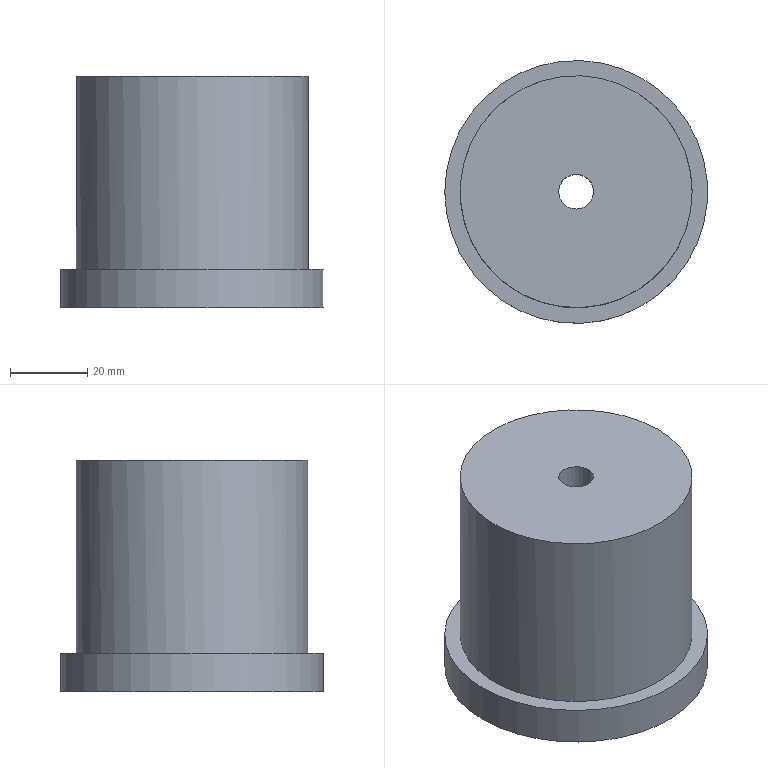Part | NX | features solid 2 | 1 solid | 8 faces | box 68 x 68 x 60 mm | volume 172968 mm3 | cylinder 4 | plane 4 | commonest cylinder face diameters 9 x1 14 x1 60 x1 68 x1
STEP:
#1=CARTESIAN_POINT('',(1081.,-600.5,-339.));
#2=VERTEX_POINT('',#1);
#3=CARTESIAN_POINT('',(1115.,-600.5,-339.));
#4=DIRECTION('',(0.,0.,-1.));
#5=DIRECTION('',(-1.,0.,0.));
#6=AXIS2_PLACEMENT_3D('',#3,#4,#5);
#7=CIRCLE('',#6,34.);
#8=EDGE_CURVE('',#2,#2,#7,.T.);
#9=ORIENTED_EDGE('',*,*,#8,.T.);
#10=EDGE_LOOP('',(#9));
#11=FACE_BOUND('',#10,.T.);
#12=CARTESIAN_POINT('',(1081.,-600.5,-349.));
#13=VERTEX_POINT('',#12);
#14=CARTESIAN_POINT('',(1115.,-600.5,-349.));
#15=DIRECTION('',(0.,0.,1.));
#16=DIRECTION('',(-1.,0.,0.));
#17=AXIS2_PLACEMENT_3D('',#14,#15,#16);
#18=CIRCLE('',#17,34.);
#19=EDGE_CURVE('',#13,#13,#18,.T.);
#20=ORIENTED_EDGE('',*,*,#19,.T.);
#21=EDGE_LOOP('',(#20));
#22=FACE_BOUND('',#21,.T.);
#23=CARTESIAN_POINT('',(1115.,-600.5,-339.));
#24=DIRECTION('',(0.,0.,-1.));
#25=DIRECTION('',(0.,-1.,0.));
#26=AXIS2_PLACEMENT_3D('',#23,#24,#25);
#27=CYLINDRICAL_SURFACE('',#26,34.);
#28=ADVANCED_FACE('',(#11,#22),#27,.T.);
#29=CARTESIAN_POINT('',(1115.,-570.5,-339.));
#30=VERTEX_POINT('',#29);
#31=CARTESIAN_POINT('',(1115.,-600.5,-339.));
#32=DIRECTION('',(0.,0.,-1.));
#33=DIRECTION('',(0.,1.,0.));
#34=AXIS2_PLACEMENT_3D('',#31,#32,#33);
#35=CIRCLE('',#34,30.);
#36=EDGE_CURVE('',#30,#30,#35,.T.);
#37=ORIENTED_EDGE('',*,*,#36,.F.);
#38=EDGE_LOOP('',(#37));
#39=FACE_BOUND('',#38,.T.);
#40=CARTESIAN_POINT('',(1145.,-600.5,-289.));
#41=VERTEX_POINT('',#40);
#42=CARTESIAN_POINT('',(1115.,-600.5,-289.));
#43=DIRECTION('',(0.,0.,-1.));
#44=DIRECTION('',(1.,0.,0.));
#45=AXIS2_PLACEMENT_3D('',#42,#43,#44);
#46=CIRCLE('',#45,30.);
#47=EDGE_CURVE('',#41,#41,#46,.T.);
#48=ORIENTED_EDGE('',*,*,#47,.T.);
#49=EDGE_LOOP('',(#48));
#50=FACE_BOUND('',#49,.T.);
#51=CARTESIAN_POINT('',(1115.,-600.5,-309.));
#52=DIRECTION('',(0.,0.,-1.));
#53=DIRECTION('',(0.,-1.,0.));
#54=AXIS2_PLACEMENT_3D('',#51,#52,#53);
#55=CYLINDRICAL_SURFACE('',#54,30.);
#56=ADVANCED_FACE('',(#39,#50),#55,.T.);
#57=ORIENTED_EDGE('',*,*,#8,.F.);
#58=EDGE_LOOP('',(#57));
#59=FACE_BOUND('',#58,.T.);
#60=ORIENTED_EDGE('',*,*,#36,.T.);
#61=EDGE_LOOP('',(#60));
#62=FACE_BOUND('',#61,.T.);
#63=CARTESIAN_POINT('',(1115.,-600.5,-339.));
#64=DIRECTION('',(0.,0.,-1.));
#65=DIRECTION('',(0.,1.,0.));
#66=AXIS2_PLACEMENT_3D('',#63,#64,#65);
#67=PLANE('',#66);
#68=ADVANCED_FACE('',(#59,#62),#67,.F.);
#69=ORIENTED_EDGE('',*,*,#19,.F.);
#70=EDGE_LOOP('',(#69));
#71=FACE_BOUND('',#70,.T.);
#72=CARTESIAN_POINT('',(1115.,-593.5,-349.));
#73=VERTEX_POINT('',#72);
#74=CARTESIAN_POINT('',(1115.,-600.5,-349.));
#75=DIRECTION('',(0.,0.,1.));
#76=DIRECTION('',(0.,1.,0.));
#77=AXIS2_PLACEMENT_3D('',#74,#75,#76);
#78=CIRCLE('',#77,7.);
#79=EDGE_CURVE('',#73,#73,#78,.T.);
#80=ORIENTED_EDGE('',*,*,#79,.T.);
#81=EDGE_LOOP('',(#80));
#82=FACE_BOUND('',#81,.T.);
#83=CARTESIAN_POINT('',(1115.,-600.5,-349.));
#84=DIRECTION('',(0.,0.,-1.));
#85=DIRECTION('',(0.,-1.,0.));
#86=AXIS2_PLACEMENT_3D('',#83,#84,#85);
#87=PLANE('',#86);
#88=ADVANCED_FACE('',(#71,#82),#87,.T.);
#89=CARTESIAN_POINT('',(1115.,-593.5,-339.));
#90=VERTEX_POINT('',#89);
#91=CARTESIAN_POINT('',(1115.,-600.5,-339.));
#92=DIRECTION('',(0.,0.,-1.));
#93=DIRECTION('',(0.,1.,0.));
#94=AXIS2_PLACEMENT_3D('',#91,#92,#93);
#95=CIRCLE('',#94,7.);
#96=EDGE_CURVE('',#90,#90,#95,.T.);
#97=ORIENTED_EDGE('',*,*,#96,.F.);
#98=EDGE_LOOP('',(#97));
#99=FACE_BOUND('',#98,.T.);
#100=ORIENTED_EDGE('',*,*,#79,.F.);
#101=EDGE_LOOP('',(#100));
#102=FACE_BOUND('',#101,.T.);
#103=CARTESIAN_POINT('',(1115.,-600.5,-339.));
#104=DIRECTION('',(0.,0.,-1.));
#105=DIRECTION('',(0.,-1.,0.));
#106=AXIS2_PLACEMENT_3D('',#103,#104,#105);
#107=CYLINDRICAL_SURFACE('',#106,7.);
#108=ADVANCED_FACE('',(#99,#102),#107,.F.);
#109=CARTESIAN_POINT('',(1115.,-596.,-339.));
#110=VERTEX_POINT('',#109);
#111=CARTESIAN_POINT('',(1115.,-600.5,-339.));
#112=DIRECTION('',(0.,0.,-1.));
#113=DIRECTION('',(0.,1.,0.));
#114=AXIS2_PLACEMENT_3D('',#111,#112,#113);
#115=CIRCLE('',#114,4.5);
#116=EDGE_CURVE('',#110,#110,#115,.T.);
#117=ORIENTED_EDGE('',*,*,#116,.F.);
#118=EDGE_LOOP('',(#117));
#119=FACE_BOUND('',#118,.T.);
#120=ORIENTED_EDGE('',*,*,#96,.T.);
#121=EDGE_LOOP('',(#120));
#122=FACE_BOUND('',#121,.T.);
#123=CARTESIAN_POINT('',(1115.,-600.5,-339.));
#124=DIRECTION('',(0.,0.,-1.));
#125=DIRECTION('',(0.,-1.,0.));
#126=AXIS2_PLACEMENT_3D('',#123,#124,#125);
#127=PLANE('',#126);
#128=ADVANCED_FACE('',(#119,#122),#127,.T.);
#129=CARTESIAN_POINT('',(1115.,-605.,-289.));
#130=VERTEX_POINT('',#129);
#131=CARTESIAN_POINT('',(1115.,-600.5,-289.));
#132=DIRECTION('',(0.,0.,1.));
#133=DIRECTION('',(0.,-1.,0.));
#134=AXIS2_PLACEMENT_3D('',#131,#132,#133);
#135=CIRCLE('',#134,4.5);
#136=EDGE_CURVE('',#130,#130,#135,.T.);
#137=ORIENTED_EDGE('',*,*,#136,.T.);
#138=EDGE_LOOP('',(#137));
#139=FACE_BOUND('',#138,.T.);
#140=ORIENTED_EDGE('',*,*,#116,.T.);
#141=EDGE_LOOP('',(#140));
#142=FACE_BOUND('',#141,.T.);
#143=CARTESIAN_POINT('',(1115.,-600.5,-314.));
#144=DIRECTION('',(0.,0.,1.));
#145=DIRECTION('',(0.,1.,0.));
#146=AXIS2_PLACEMENT_3D('',#143,#144,#145);
#147=CYLINDRICAL_SURFACE('',#146,4.5);
#148=ADVANCED_FACE('',(#139,#142),#147,.F.);
#149=ORIENTED_EDGE('',*,*,#47,.F.);
#150=EDGE_LOOP('',(#149));
#151=FACE_BOUND('',#150,.T.);
#152=ORIENTED_EDGE('',*,*,#136,.F.);
#153=EDGE_LOOP('',(#152));
#154=FACE_BOUND('',#153,.T.);
#155=CARTESIAN_POINT('',(1115.,-566.,-289.));
#156=DIRECTION('',(0.,0.,1.));
#157=DIRECTION('',(0.,1.,0.));
#158=AXIS2_PLACEMENT_3D('',#155,#156,#157);
#159=PLANE('',#158);
#160=ADVANCED_FACE('',(#151,#154),#159,.T.);
#161=CLOSED_SHELL('',(#28,#56,#68,#88,#108,#128,#148,#160));
#162=MANIFOLD_SOLID_BREP('',#161);
#163=(LENGTH_UNIT()NAMED_UNIT(*)SI_UNIT(.MILLI.,.METRE.));
#164=UNCERTAINTY_MEASURE_WITH_UNIT(LENGTH_MEASURE(0.00001),#163,'','');
#165=(NAMED_UNIT(*)PLANE_ANGLE_UNIT()SI_UNIT($,.RADIAN.));
#166=(NAMED_UNIT(*)SI_UNIT($,.STERADIAN.)SOLID_ANGLE_UNIT());
#167=(GEOMETRIC_REPRESENTATION_CONTEXT(3)GLOBAL_UNCERTAINTY_ASSIGNED_CONTEXT((#164))GLOBAL_UNIT_ASSIGNED_CONTEXT((#163,#165,#166))REPRESENTATION_CONTEXT('',''));
#168=ADVANCED_BREP_SHAPE_REPRESENTATION('',(#162),#167);